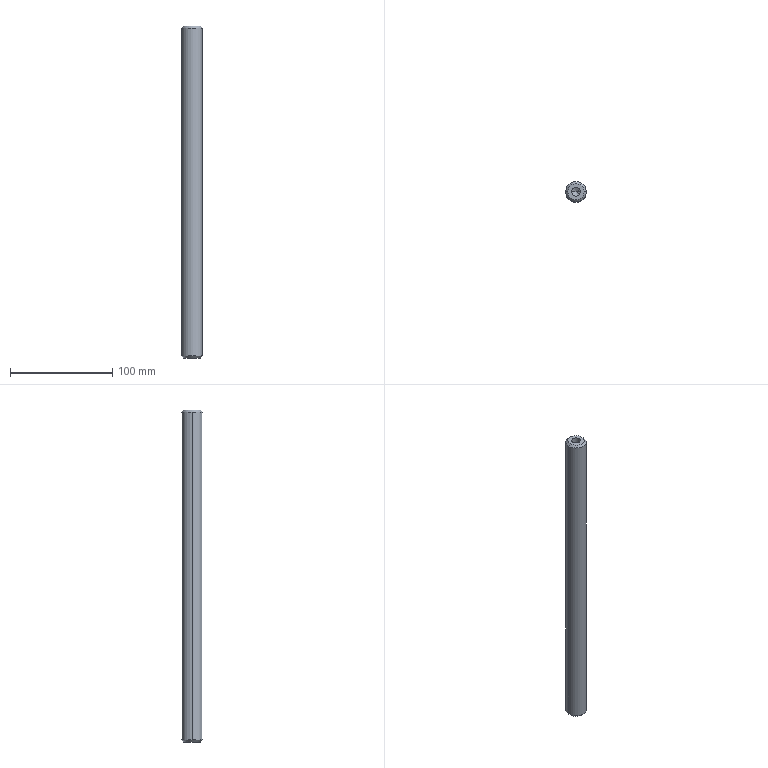Part | SolidWorks | features HoleWzd 2, Chamfer 1, Extrusion 1 | 1 solid | 16 faces | box 20 x 20 x 324 mm | volume 98619 mm3 | cone 8 | cylinder 6 | plane 2 | commonest cylinder face diameters 8.5 x4 20 x2
STEP:
#1=CARTESIAN_POINT('',(4.25,0.,-137.));
#2=VERTEX_POINT('',#1);
#3=CARTESIAN_POINT('',(-4.25,0.,-137.));
#4=VERTEX_POINT('',#3);
#5=CARTESIAN_POINT('',(0.,0.,-137.));
#6=DIRECTION('',(0.,0.,-1.));
#7=DIRECTION('',(-1.,0.,0.));
#8=AXIS2_PLACEMENT_3D('',#5,#6,#7);
#9=CIRCLE('',#8,4.25);
#10=EDGE_CURVE('',#2,#4,#9,.T.);
#11=ORIENTED_EDGE('',*,*,#10,.F.);
#12=CARTESIAN_POINT('',(4.25,0.,-162.));
#13=VERTEX_POINT('',#12);
#14=CARTESIAN_POINT('',(4.25,0.,-162.));
#15=DIRECTION('',(0.,0.,-1.));
#16=VECTOR('',#15,1000.);
#17=LINE('',#14,#16);
#18=EDGE_CURVE('',#2,#13,#17,.T.);
#19=ORIENTED_EDGE('',*,*,#18,.T.);
#20=CARTESIAN_POINT('',(-4.25,0.,-162.));
#21=VERTEX_POINT('',#20);
#22=CARTESIAN_POINT('',(0.,0.,-162.));
#23=DIRECTION('',(0.,0.,-1.));
#24=DIRECTION('',(-1.,0.,0.));
#25=AXIS2_PLACEMENT_3D('',#22,#23,#24);
#26=CIRCLE('',#25,4.25);
#27=EDGE_CURVE('',#13,#21,#26,.T.);
#28=ORIENTED_EDGE('',*,*,#27,.T.);
#29=CARTESIAN_POINT('',(-4.25,0.,-162.));
#30=DIRECTION('',(0.,0.,-1.));
#31=VECTOR('',#30,1000.);
#32=LINE('',#29,#31);
#33=EDGE_CURVE('',#4,#21,#32,.T.);
#34=ORIENTED_EDGE('',*,*,#33,.F.);
#35=EDGE_LOOP('',(#11,#19,#28,#34));
#36=FACE_OUTER_BOUND('',#35,.T.);
#37=CARTESIAN_POINT('',(0.,0.,-162.));
#38=DIRECTION('',(0.,0.,-1.));
#39=DIRECTION('',(-1.,0.,0.));
#40=AXIS2_PLACEMENT_3D('',#37,#38,#39);
#41=CYLINDRICAL_SURFACE('',#40,4.25);
#42=ADVANCED_FACE('',(#36),#41,.F.);
#43=CARTESIAN_POINT('',(0.,0.,-134.446));
#44=VERTEX_POINT('',#43);
#45=CARTESIAN_POINT('',(-4.25,0.,-137.));
#46=DIRECTION('',(-0.8572,0.,-0.515));
#47=VECTOR('',#46,1000.);
#48=LINE('',#45,#47);
#49=EDGE_CURVE('',#44,#4,#48,.T.);
#50=ORIENTED_EDGE('',*,*,#49,.F.);
#51=CARTESIAN_POINT('',(4.25,0.,-137.));
#52=DIRECTION('',(0.8572,0.,-0.515));
#53=VECTOR('',#52,1000.);
#54=LINE('',#51,#53);
#55=EDGE_CURVE('',#44,#2,#54,.T.);
#56=ORIENTED_EDGE('',*,*,#55,.T.);
#57=ORIENTED_EDGE('',*,*,#10,.T.);
#58=EDGE_LOOP('',(#50,#56,#57));
#59=FACE_OUTER_BOUND('',#58,.T.);
#60=CARTESIAN_POINT('',(0.,0.,-137.));
#61=DIRECTION('',(0.,0.,-1.));
#62=DIRECTION('',(-1.,0.,0.));
#63=AXIS2_PLACEMENT_3D('',#60,#61,#62);
#64=CONICAL_SURFACE('',#63,4.25,1.03);
#65=ADVANCED_FACE('',(#59),#64,.F.);
#66=CARTESIAN_POINT('',(-4.25,0.,137.));
#67=VERTEX_POINT('',#66);
#68=CARTESIAN_POINT('',(4.25,0.,137.));
#69=VERTEX_POINT('',#68);
#70=CARTESIAN_POINT('',(0.,0.,137.));
#71=DIRECTION('',(0.,0.,1.));
#72=DIRECTION('',(1.,0.,0.));
#73=AXIS2_PLACEMENT_3D('',#70,#71,#72);
#74=CIRCLE('',#73,4.25);
#75=EDGE_CURVE('',#67,#69,#74,.T.);
#76=ORIENTED_EDGE('',*,*,#75,.F.);
#77=CARTESIAN_POINT('',(-4.25,0.,162.));
#78=VERTEX_POINT('',#77);
#79=CARTESIAN_POINT('',(-4.25,0.,162.));
#80=DIRECTION('',(0.,0.,1.));
#81=VECTOR('',#80,1000.);
#82=LINE('',#79,#81);
#83=EDGE_CURVE('',#67,#78,#82,.T.);
#84=ORIENTED_EDGE('',*,*,#83,.T.);
#85=CARTESIAN_POINT('',(4.25,0.,162.));
#86=VERTEX_POINT('',#85);
#87=CARTESIAN_POINT('',(0.,0.,162.));
#88=DIRECTION('',(0.,0.,1.));
#89=DIRECTION('',(1.,0.,0.));
#90=AXIS2_PLACEMENT_3D('',#87,#88,#89);
#91=CIRCLE('',#90,4.25);
#92=EDGE_CURVE('',#78,#86,#91,.T.);
#93=ORIENTED_EDGE('',*,*,#92,.T.);
#94=CARTESIAN_POINT('',(4.25,0.,162.));
#95=DIRECTION('',(0.,0.,1.));
#96=VECTOR('',#95,1000.);
#97=LINE('',#94,#96);
#98=EDGE_CURVE('',#69,#86,#97,.T.);
#99=ORIENTED_EDGE('',*,*,#98,.F.);
#100=EDGE_LOOP('',(#76,#84,#93,#99));
#101=FACE_OUTER_BOUND('',#100,.T.);
#102=CARTESIAN_POINT('',(0.,0.,162.));
#103=DIRECTION('',(0.,0.,1.));
#104=DIRECTION('',(1.,0.,0.));
#105=AXIS2_PLACEMENT_3D('',#102,#103,#104);
#106=CYLINDRICAL_SURFACE('',#105,4.25);
#107=ADVANCED_FACE('',(#101),#106,.F.);
#108=CARTESIAN_POINT('',(0.,0.,134.446));
#109=VERTEX_POINT('',#108);
#110=CARTESIAN_POINT('',(4.25,0.,137.));
#111=DIRECTION('',(0.8572,0.,0.515));
#112=VECTOR('',#111,1000.);
#113=LINE('',#110,#112);
#114=EDGE_CURVE('',#109,#69,#113,.T.);
#115=ORIENTED_EDGE('',*,*,#114,.F.);
#116=CARTESIAN_POINT('',(-4.25,0.,137.));
#117=DIRECTION('',(-0.8572,0.,0.515));
#118=VECTOR('',#117,1000.);
#119=LINE('',#116,#118);
#120=EDGE_CURVE('',#109,#67,#119,.T.);
#121=ORIENTED_EDGE('',*,*,#120,.T.);
#122=ORIENTED_EDGE('',*,*,#75,.T.);
#123=EDGE_LOOP('',(#115,#121,#122));
#124=FACE_OUTER_BOUND('',#123,.T.);
#125=CARTESIAN_POINT('',(0.,0.,137.));
#126=DIRECTION('',(0.,0.,1.));
#127=DIRECTION('',(1.,0.,0.));
#128=AXIS2_PLACEMENT_3D('',#125,#126,#127);
#129=CONICAL_SURFACE('',#128,4.25,1.03);
#130=ADVANCED_FACE('',(#124),#129,.F.);
#131=CARTESIAN_POINT('',(8.,0.,162.));
#132=VERTEX_POINT('',#131);
#133=CARTESIAN_POINT('',(-8.,0.,162.));
#134=VERTEX_POINT('',#133);
#135=CARTESIAN_POINT('',(0.,0.,162.));
#136=DIRECTION('',(0.,0.,1.));
#137=DIRECTION('',(1.,0.,0.));
#138=AXIS2_PLACEMENT_3D('',#135,#136,#137);
#139=CIRCLE('',#138,8.);
#140=EDGE_CURVE('',#132,#134,#139,.T.);
#141=ORIENTED_EDGE('',*,*,#140,.F.);
#142=CARTESIAN_POINT('',(10.,0.,160.));
#143=VERTEX_POINT('',#142);
#144=CARTESIAN_POINT('',(8.,0.,162.));
#145=DIRECTION('',(0.7071,0.,-0.7071));
#146=VECTOR('',#145,1000.);
#147=LINE('',#144,#146);
#148=EDGE_CURVE('',#132,#143,#147,.T.);
#149=ORIENTED_EDGE('',*,*,#148,.T.);
#150=CARTESIAN_POINT('',(-10.,0.,160.));
#151=VERTEX_POINT('',#150);
#152=CARTESIAN_POINT('',(0.,0.,160.));
#153=DIRECTION('',(0.,0.,-1.));
#154=DIRECTION('',(1.,0.,0.));
#155=AXIS2_PLACEMENT_3D('',#152,#153,#154);
#156=CIRCLE('',#155,10.);
#157=EDGE_CURVE('',#151,#143,#156,.T.);
#158=ORIENTED_EDGE('',*,*,#157,.F.);
#159=CARTESIAN_POINT('',(-8.,0.,162.));
#160=DIRECTION('',(-0.7071,0.,-0.7071));
#161=VECTOR('',#160,1000.);
#162=LINE('',#159,#161);
#163=EDGE_CURVE('',#134,#151,#162,.T.);
#164=ORIENTED_EDGE('',*,*,#163,.F.);
#165=EDGE_LOOP('',(#141,#149,#158,#164));
#166=FACE_OUTER_BOUND('',#165,.T.);
#167=CARTESIAN_POINT('',(0.,0.,162.));
#168=DIRECTION('',(0.,0.,-1.));
#169=DIRECTION('',(-1.,0.,0.));
#170=AXIS2_PLACEMENT_3D('',#167,#168,#169);
#171=CONICAL_SURFACE('',#170,8.,0.7854);
#172=ADVANCED_FACE('',(#166),#171,.T.);
#173=CARTESIAN_POINT('',(-8.,0.,-162.));
#174=VERTEX_POINT('',#173);
#175=CARTESIAN_POINT('',(8.,0.,-162.));
#176=VERTEX_POINT('',#175);
#177=CARTESIAN_POINT('',(0.,0.,-162.));
#178=DIRECTION('',(0.,0.,-1.));
#179=DIRECTION('',(1.,0.,0.));
#180=AXIS2_PLACEMENT_3D('',#177,#178,#179);
#181=CIRCLE('',#180,8.);
#182=EDGE_CURVE('',#174,#176,#181,.T.);
#183=ORIENTED_EDGE('',*,*,#182,.F.);
#184=CARTESIAN_POINT('',(-10.,0.,-160.));
#185=VERTEX_POINT('',#184);
#186=CARTESIAN_POINT('',(-10.,0.,-160.));
#187=DIRECTION('',(-0.7071,0.,0.7071));
#188=VECTOR('',#187,1000.);
#189=LINE('',#186,#188);
#190=EDGE_CURVE('',#174,#185,#189,.T.);
#191=ORIENTED_EDGE('',*,*,#190,.T.);
#192=CARTESIAN_POINT('',(10.,0.,-160.));
#193=VERTEX_POINT('',#192);
#194=CARTESIAN_POINT('',(0.,0.,-160.));
#195=DIRECTION('',(0.,0.,1.));
#196=DIRECTION('',(1.,0.,0.));
#197=AXIS2_PLACEMENT_3D('',#194,#195,#196);
#198=CIRCLE('',#197,10.);
#199=EDGE_CURVE('',#193,#185,#198,.T.);
#200=ORIENTED_EDGE('',*,*,#199,.F.);
#201=CARTESIAN_POINT('',(10.,0.,-160.));
#202=DIRECTION('',(0.7071,0.,0.7071));
#203=VECTOR('',#202,1000.);
#204=LINE('',#201,#203);
#205=EDGE_CURVE('',#176,#193,#204,.T.);
#206=ORIENTED_EDGE('',*,*,#205,.F.);
#207=EDGE_LOOP('',(#183,#191,#200,#206));
#208=FACE_OUTER_BOUND('',#207,.T.);
#209=CARTESIAN_POINT('',(0.,0.,-160.));
#210=DIRECTION('',(0.,0.,1.));
#211=DIRECTION('',(1.,0.,0.));
#212=AXIS2_PLACEMENT_3D('',#209,#210,#211);
#213=CONICAL_SURFACE('',#212,10.,0.7854);
#214=ADVANCED_FACE('',(#208),#213,.T.);
#215=ORIENTED_EDGE('',*,*,#157,.T.);
#216=CARTESIAN_POINT('',(10.,0.,162.));
#217=DIRECTION('',(0.,0.,-1.));
#218=VECTOR('',#217,1000.);
#219=LINE('',#216,#218);
#220=EDGE_CURVE('',#143,#193,#219,.T.);
#221=ORIENTED_EDGE('',*,*,#220,.T.);
#222=ORIENTED_EDGE('',*,*,#199,.T.);
#223=CARTESIAN_POINT('',(-10.,0.,162.));
#224=DIRECTION('',(0.,0.,-1.));
#225=VECTOR('',#224,1000.);
#226=LINE('',#223,#225);
#227=EDGE_CURVE('',#151,#185,#226,.T.);
#228=ORIENTED_EDGE('',*,*,#227,.F.);
#229=EDGE_LOOP('',(#215,#221,#222,#228));
#230=FACE_OUTER_BOUND('',#229,.T.);
#231=CARTESIAN_POINT('',(0.,0.,162.));
#232=DIRECTION('',(0.,0.,-1.));
#233=DIRECTION('',(-1.,0.,0.));
#234=AXIS2_PLACEMENT_3D('',#231,#232,#233);
#235=CYLINDRICAL_SURFACE('',#234,10.);
#236=ADVANCED_FACE('',(#230),#235,.T.);
#237=ORIENTED_EDGE('',*,*,#220,.F.);
#238=CARTESIAN_POINT('',(0.,0.,160.));
#239=DIRECTION('',(0.,0.,-1.));
#240=DIRECTION('',(1.,0.,0.));
#241=AXIS2_PLACEMENT_3D('',#238,#239,#240);
#242=CIRCLE('',#241,10.);
#243=EDGE_CURVE('',#143,#151,#242,.T.);
#244=ORIENTED_EDGE('',*,*,#243,.T.);
#245=ORIENTED_EDGE('',*,*,#227,.T.);
#246=CARTESIAN_POINT('',(0.,0.,-160.));
#247=DIRECTION('',(0.,0.,1.));
#248=DIRECTION('',(1.,0.,0.));
#249=AXIS2_PLACEMENT_3D('',#246,#247,#248);
#250=CIRCLE('',#249,10.);
#251=EDGE_CURVE('',#185,#193,#250,.T.);
#252=ORIENTED_EDGE('',*,*,#251,.T.);
#253=EDGE_LOOP('',(#237,#244,#245,#252));
#254=FACE_OUTER_BOUND('',#253,.T.);
#255=CARTESIAN_POINT('',(0.,0.,162.));
#256=DIRECTION('',(0.,0.,-1.));
#257=DIRECTION('',(-1.,0.,0.));
#258=AXIS2_PLACEMENT_3D('',#255,#256,#257);
#259=CYLINDRICAL_SURFACE('',#258,10.);
#260=ADVANCED_FACE('',(#254),#259,.T.);
#261=CARTESIAN_POINT('',(0.,0.,162.));
#262=DIRECTION('',(0.,0.,1.));
#263=DIRECTION('',(1.,0.,0.));
#264=AXIS2_PLACEMENT_3D('',#261,#262,#263);
#265=CIRCLE('',#264,4.25);
#266=EDGE_CURVE('',#86,#78,#265,.T.);
#267=ORIENTED_EDGE('',*,*,#266,.F.);
#268=ORIENTED_EDGE('',*,*,#92,.F.);
#269=EDGE_LOOP('',(#267,#268));
#270=FACE_BOUND('',#269,.T.);
#271=CARTESIAN_POINT('',(0.,0.,162.));
#272=DIRECTION('',(0.,0.,1.));
#273=DIRECTION('',(1.,0.,0.));
#274=AXIS2_PLACEMENT_3D('',#271,#272,#273);
#275=CIRCLE('',#274,8.);
#276=EDGE_CURVE('',#134,#132,#275,.T.);
#277=ORIENTED_EDGE('',*,*,#276,.T.);
#278=ORIENTED_EDGE('',*,*,#140,.T.);
#279=EDGE_LOOP('',(#277,#278));
#280=FACE_OUTER_BOUND('',#279,.T.);
#281=CARTESIAN_POINT('',(0.,0.,162.));
#282=DIRECTION('',(0.,0.,1.));
#283=DIRECTION('',(1.,0.,0.));
#284=AXIS2_PLACEMENT_3D('',#281,#282,#283);
#285=PLANE('',#284);
#286=ADVANCED_FACE('',(#270,#280),#285,.T.);
#287=CARTESIAN_POINT('',(0.,0.,-162.));
#288=DIRECTION('',(0.,0.,-1.));
#289=DIRECTION('',(-1.,0.,0.));
#290=AXIS2_PLACEMENT_3D('',#287,#288,#289);
#291=CIRCLE('',#290,4.25);
#292=EDGE_CURVE('',#21,#13,#291,.T.);
#293=ORIENTED_EDGE('',*,*,#292,.F.);
#294=ORIENTED_EDGE('',*,*,#27,.F.);
#295=EDGE_LOOP('',(#293,#294));
#296=FACE_BOUND('',#295,.T.);
#297=CARTESIAN_POINT('',(0.,0.,-162.));
#298=DIRECTION('',(0.,0.,-1.));
#299=DIRECTION('',(1.,0.,0.));
#300=AXIS2_PLACEMENT_3D('',#297,#298,#299);
#301=CIRCLE('',#300,8.);
#302=EDGE_CURVE('',#176,#174,#301,.T.);
#303=ORIENTED_EDGE('',*,*,#302,.T.);
#304=ORIENTED_EDGE('',*,*,#182,.T.);
#305=EDGE_LOOP('',(#303,#304));
#306=FACE_OUTER_BOUND('',#305,.T.);
#307=CARTESIAN_POINT('',(0.,0.,-162.));
#308=DIRECTION('',(0.,0.,1.));
#309=DIRECTION('',(1.,0.,0.));
#310=AXIS2_PLACEMENT_3D('',#307,#308,#309);
#311=PLANE('',#310);
#312=ADVANCED_FACE('',(#296,#306),#311,.F.);
#313=ORIENTED_EDGE('',*,*,#190,.F.);
#314=ORIENTED_EDGE('',*,*,#302,.F.);
#315=ORIENTED_EDGE('',*,*,#205,.T.);
#316=ORIENTED_EDGE('',*,*,#251,.F.);
#317=EDGE_LOOP('',(#313,#314,#315,#316));
#318=FACE_OUTER_BOUND('',#317,.T.);
#319=CARTESIAN_POINT('',(0.,0.,-160.));
#320=DIRECTION('',(0.,0.,1.));
#321=DIRECTION('',(1.,0.,0.));
#322=AXIS2_PLACEMENT_3D('',#319,#320,#321);
#323=CONICAL_SURFACE('',#322,10.,0.7854);
#324=ADVANCED_FACE('',(#318),#323,.T.);
#325=ORIENTED_EDGE('',*,*,#148,.F.);
#326=ORIENTED_EDGE('',*,*,#276,.F.);
#327=ORIENTED_EDGE('',*,*,#163,.T.);
#328=ORIENTED_EDGE('',*,*,#243,.F.);
#329=EDGE_LOOP('',(#325,#326,#327,#328));
#330=FACE_OUTER_BOUND('',#329,.T.);
#331=CARTESIAN_POINT('',(0.,0.,162.));
#332=DIRECTION('',(0.,0.,-1.));
#333=DIRECTION('',(-1.,0.,0.));
#334=AXIS2_PLACEMENT_3D('',#331,#332,#333);
#335=CONICAL_SURFACE('',#334,8.,0.7854);
#336=ADVANCED_FACE('',(#330),#335,.T.);
#337=ORIENTED_EDGE('',*,*,#120,.F.);
#338=ORIENTED_EDGE('',*,*,#114,.T.);
#339=CARTESIAN_POINT('',(0.,0.,137.));
#340=DIRECTION('',(0.,0.,1.));
#341=DIRECTION('',(1.,0.,0.));
#342=AXIS2_PLACEMENT_3D('',#339,#340,#341);
#343=CIRCLE('',#342,4.25);
#344=EDGE_CURVE('',#69,#67,#343,.T.);
#345=ORIENTED_EDGE('',*,*,#344,.T.);
#346=EDGE_LOOP('',(#337,#338,#345));
#347=FACE_OUTER_BOUND('',#346,.T.);
#348=CARTESIAN_POINT('',(0.,0.,137.));
#349=DIRECTION('',(0.,0.,1.));
#350=DIRECTION('',(1.,0.,0.));
#351=AXIS2_PLACEMENT_3D('',#348,#349,#350);
#352=CONICAL_SURFACE('',#351,4.25,1.03);
#353=ADVANCED_FACE('',(#347),#352,.F.);
#354=ORIENTED_EDGE('',*,*,#83,.F.);
#355=ORIENTED_EDGE('',*,*,#344,.F.);
#356=ORIENTED_EDGE('',*,*,#98,.T.);
#357=ORIENTED_EDGE('',*,*,#266,.T.);
#358=EDGE_LOOP('',(#354,#355,#356,#357));
#359=FACE_OUTER_BOUND('',#358,.T.);
#360=CARTESIAN_POINT('',(0.,0.,162.));
#361=DIRECTION('',(0.,0.,1.));
#362=DIRECTION('',(1.,0.,0.));
#363=AXIS2_PLACEMENT_3D('',#360,#361,#362);
#364=CYLINDRICAL_SURFACE('',#363,4.25);
#365=ADVANCED_FACE('',(#359),#364,.F.);
#366=ORIENTED_EDGE('',*,*,#55,.F.);
#367=ORIENTED_EDGE('',*,*,#49,.T.);
#368=CARTESIAN_POINT('',(0.,0.,-137.));
#369=DIRECTION('',(0.,0.,-1.));
#370=DIRECTION('',(-1.,0.,0.));
#371=AXIS2_PLACEMENT_3D('',#368,#369,#370);
#372=CIRCLE('',#371,4.25);
#373=EDGE_CURVE('',#4,#2,#372,.T.);
#374=ORIENTED_EDGE('',*,*,#373,.T.);
#375=EDGE_LOOP('',(#366,#367,#374));
#376=FACE_OUTER_BOUND('',#375,.T.);
#377=CARTESIAN_POINT('',(0.,0.,-137.));
#378=DIRECTION('',(0.,0.,-1.));
#379=DIRECTION('',(-1.,0.,0.));
#380=AXIS2_PLACEMENT_3D('',#377,#378,#379);
#381=CONICAL_SURFACE('',#380,4.25,1.03);
#382=ADVANCED_FACE('',(#376),#381,.F.);
#383=ORIENTED_EDGE('',*,*,#18,.F.);
#384=ORIENTED_EDGE('',*,*,#373,.F.);
#385=ORIENTED_EDGE('',*,*,#33,.T.);
#386=ORIENTED_EDGE('',*,*,#292,.T.);
#387=EDGE_LOOP('',(#383,#384,#385,#386));
#388=FACE_OUTER_BOUND('',#387,.T.);
#389=CARTESIAN_POINT('',(0.,0.,-162.));
#390=DIRECTION('',(0.,0.,-1.));
#391=DIRECTION('',(-1.,0.,0.));
#392=AXIS2_PLACEMENT_3D('',#389,#390,#391);
#393=CYLINDRICAL_SURFACE('',#392,4.25);
#394=ADVANCED_FACE('',(#388),#393,.F.);
#395=CLOSED_SHELL('',(#42,#65,#107,#130,#172,#214,#236,#260,#286,#312,#324,#336,#353,#365,#382,#394));
#396=MANIFOLD_SOLID_BREP('',#395);
#397=CARTESIAN_POINT('',(0.,0.,0.));
#398=DIRECTION('',(0.,0.,1.));
#399=DIRECTION('',(1.,0.,0.));
#400=AXIS2_PLACEMENT_3D('',#397,#398,#399);
#401=(LENGTH_UNIT()NAMED_UNIT(*)SI_UNIT(.MILLI.,.METRE.));
#402=UNCERTAINTY_MEASURE_WITH_UNIT(LENGTH_MEASURE(0.00001),#401,'','');
#403=(NAMED_UNIT(*)PLANE_ANGLE_UNIT()SI_UNIT($,.RADIAN.));
#404=(NAMED_UNIT(*)SI_UNIT($,.STERADIAN.)SOLID_ANGLE_UNIT());
#405=(GEOMETRIC_REPRESENTATION_CONTEXT(3)GLOBAL_UNCERTAINTY_ASSIGNED_CONTEXT((#402))GLOBAL_UNIT_ASSIGNED_CONTEXT((#401,#403,#404))REPRESENTATION_CONTEXT('',''));
#406=ADVANCED_BREP_SHAPE_REPRESENTATION('',(#396,#400),#405);